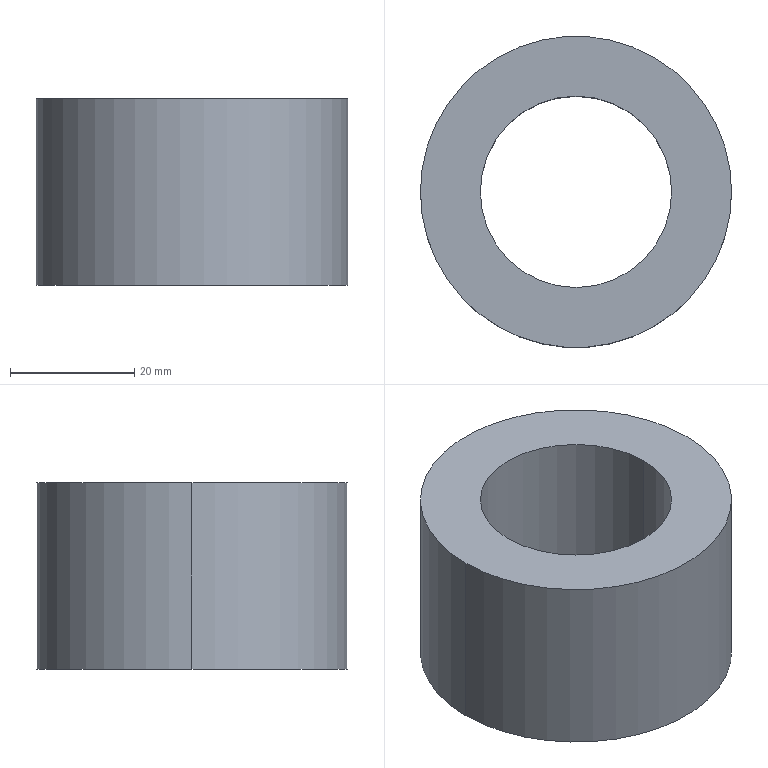Part | SolidWorks | features 3DProfileFeature 1, Extrusion 1, HoleWzd 1 | 1 solid | 6 faces | box 50 x 50 x 30 mm | volume 36626 mm3 | cylinder 4 | plane 2 | commonest cylinder face diameters 30.75 x2 50 x2
STEP:
#1=CARTESIAN_POINT('',(15.375,0.,30.));
#2=VERTEX_POINT('',#1);
#3=CARTESIAN_POINT('',(-15.375,0.,30.));
#4=VERTEX_POINT('',#3);
#5=CARTESIAN_POINT('',(0.,0.,30.));
#6=DIRECTION('',(0.,0.,-1.));
#7=DIRECTION('',(-1.,0.,0.));
#8=AXIS2_PLACEMENT_3D('',#5,#6,#7);
#9=CIRCLE('',#8,15.375);
#10=EDGE_CURVE('',#2,#4,#9,.T.);
#11=ORIENTED_EDGE('',*,*,#10,.F.);
#12=CARTESIAN_POINT('',(15.375,0.,0.));
#13=VERTEX_POINT('',#12);
#14=CARTESIAN_POINT('',(15.375,0.,0.));
#15=DIRECTION('',(0.,0.,-1.));
#16=VECTOR('',#15,1000.);
#17=LINE('',#14,#16);
#18=EDGE_CURVE('',#2,#13,#17,.T.);
#19=ORIENTED_EDGE('',*,*,#18,.T.);
#20=CARTESIAN_POINT('',(-15.375,0.,0.));
#21=VERTEX_POINT('',#20);
#22=CARTESIAN_POINT('',(0.,0.,0.));
#23=DIRECTION('',(0.,0.,-1.));
#24=DIRECTION('',(-1.,0.,0.));
#25=AXIS2_PLACEMENT_3D('',#22,#23,#24);
#26=CIRCLE('',#25,15.375);
#27=EDGE_CURVE('',#13,#21,#26,.T.);
#28=ORIENTED_EDGE('',*,*,#27,.T.);
#29=CARTESIAN_POINT('',(-15.375,0.,0.));
#30=DIRECTION('',(0.,0.,-1.));
#31=VECTOR('',#30,1000.);
#32=LINE('',#29,#31);
#33=EDGE_CURVE('',#4,#21,#32,.T.);
#34=ORIENTED_EDGE('',*,*,#33,.F.);
#35=EDGE_LOOP('',(#11,#19,#28,#34));
#36=FACE_OUTER_BOUND('',#35,.T.);
#37=CARTESIAN_POINT('',(0.,0.,0.));
#38=DIRECTION('',(0.,0.,-1.));
#39=DIRECTION('',(-1.,0.,0.));
#40=AXIS2_PLACEMENT_3D('',#37,#38,#39);
#41=CYLINDRICAL_SURFACE('',#40,15.375);
#42=ADVANCED_FACE('',(#36),#41,.F.);
#43=CARTESIAN_POINT('',(25.,0.,30.));
#44=VERTEX_POINT('',#43);
#45=CARTESIAN_POINT('',(-25.,0.,30.));
#46=VERTEX_POINT('',#45);
#47=CARTESIAN_POINT('',(0.,0.,30.));
#48=DIRECTION('',(0.,0.,1.));
#49=DIRECTION('',(1.,0.,0.));
#50=AXIS2_PLACEMENT_3D('',#47,#48,#49);
#51=CIRCLE('',#50,25.);
#52=EDGE_CURVE('',#44,#46,#51,.T.);
#53=ORIENTED_EDGE('',*,*,#52,.F.);
#54=CARTESIAN_POINT('',(25.,0.,0.));
#55=VERTEX_POINT('',#54);
#56=CARTESIAN_POINT('',(25.,0.,30.));
#57=DIRECTION('',(0.,0.,-1.));
#58=VECTOR('',#57,1000.);
#59=LINE('',#56,#58);
#60=EDGE_CURVE('',#44,#55,#59,.T.);
#61=ORIENTED_EDGE('',*,*,#60,.T.);
#62=CARTESIAN_POINT('',(-25.,0.,0.));
#63=VERTEX_POINT('',#62);
#64=CARTESIAN_POINT('',(0.,0.,0.));
#65=DIRECTION('',(0.,0.,1.));
#66=DIRECTION('',(1.,0.,0.));
#67=AXIS2_PLACEMENT_3D('',#64,#65,#66);
#68=CIRCLE('',#67,25.);
#69=EDGE_CURVE('',#55,#63,#68,.T.);
#70=ORIENTED_EDGE('',*,*,#69,.T.);
#71=CARTESIAN_POINT('',(-25.,0.,30.));
#72=DIRECTION('',(0.,0.,-1.));
#73=VECTOR('',#72,1000.);
#74=LINE('',#71,#73);
#75=EDGE_CURVE('',#46,#63,#74,.T.);
#76=ORIENTED_EDGE('',*,*,#75,.F.);
#77=EDGE_LOOP('',(#53,#61,#70,#76));
#78=FACE_OUTER_BOUND('',#77,.T.);
#79=CARTESIAN_POINT('',(0.,0.,30.));
#80=DIRECTION('',(0.,0.,-1.));
#81=DIRECTION('',(-1.,0.,0.));
#82=AXIS2_PLACEMENT_3D('',#79,#80,#81);
#83=CYLINDRICAL_SURFACE('',#82,25.);
#84=ADVANCED_FACE('',(#78),#83,.T.);
#85=ORIENTED_EDGE('',*,*,#60,.F.);
#86=CARTESIAN_POINT('',(0.,0.,30.));
#87=DIRECTION('',(0.,0.,1.));
#88=DIRECTION('',(1.,0.,0.));
#89=AXIS2_PLACEMENT_3D('',#86,#87,#88);
#90=CIRCLE('',#89,25.);
#91=EDGE_CURVE('',#46,#44,#90,.T.);
#92=ORIENTED_EDGE('',*,*,#91,.F.);
#93=ORIENTED_EDGE('',*,*,#75,.T.);
#94=CARTESIAN_POINT('',(0.,0.,0.));
#95=DIRECTION('',(0.,0.,1.));
#96=DIRECTION('',(1.,0.,0.));
#97=AXIS2_PLACEMENT_3D('',#94,#95,#96);
#98=CIRCLE('',#97,25.);
#99=EDGE_CURVE('',#63,#55,#98,.T.);
#100=ORIENTED_EDGE('',*,*,#99,.T.);
#101=EDGE_LOOP('',(#85,#92,#93,#100));
#102=FACE_OUTER_BOUND('',#101,.T.);
#103=CARTESIAN_POINT('',(0.,0.,30.));
#104=DIRECTION('',(0.,0.,-1.));
#105=DIRECTION('',(-1.,0.,0.));
#106=AXIS2_PLACEMENT_3D('',#103,#104,#105);
#107=CYLINDRICAL_SURFACE('',#106,25.);
#108=ADVANCED_FACE('',(#102),#107,.T.);
#109=CARTESIAN_POINT('',(0.,0.,30.));
#110=DIRECTION('',(0.,0.,-1.));
#111=DIRECTION('',(-1.,0.,0.));
#112=AXIS2_PLACEMENT_3D('',#109,#110,#111);
#113=CIRCLE('',#112,15.375);
#114=EDGE_CURVE('',#4,#2,#113,.T.);
#115=ORIENTED_EDGE('',*,*,#114,.T.);
#116=ORIENTED_EDGE('',*,*,#10,.T.);
#117=EDGE_LOOP('',(#115,#116));
#118=FACE_BOUND('',#117,.T.);
#119=ORIENTED_EDGE('',*,*,#91,.T.);
#120=ORIENTED_EDGE('',*,*,#52,.T.);
#121=EDGE_LOOP('',(#119,#120));
#122=FACE_OUTER_BOUND('',#121,.T.);
#123=CARTESIAN_POINT('',(0.,0.,30.));
#124=DIRECTION('',(0.,0.,1.));
#125=DIRECTION('',(1.,0.,0.));
#126=AXIS2_PLACEMENT_3D('',#123,#124,#125);
#127=PLANE('',#126);
#128=ADVANCED_FACE('',(#118,#122),#127,.T.);
#129=CARTESIAN_POINT('',(0.,0.,0.));
#130=DIRECTION('',(0.,0.,-1.));
#131=DIRECTION('',(-1.,0.,0.));
#132=AXIS2_PLACEMENT_3D('',#129,#130,#131);
#133=CIRCLE('',#132,15.375);
#134=EDGE_CURVE('',#21,#13,#133,.T.);
#135=ORIENTED_EDGE('',*,*,#134,.F.);
#136=ORIENTED_EDGE('',*,*,#27,.F.);
#137=EDGE_LOOP('',(#135,#136));
#138=FACE_BOUND('',#137,.T.);
#139=ORIENTED_EDGE('',*,*,#99,.F.);
#140=ORIENTED_EDGE('',*,*,#69,.F.);
#141=EDGE_LOOP('',(#139,#140));
#142=FACE_OUTER_BOUND('',#141,.T.);
#143=CARTESIAN_POINT('',(0.,0.,0.));
#144=DIRECTION('',(0.,0.,1.));
#145=DIRECTION('',(1.,0.,0.));
#146=AXIS2_PLACEMENT_3D('',#143,#144,#145);
#147=PLANE('',#146);
#148=ADVANCED_FACE('',(#138,#142),#147,.F.);
#149=ORIENTED_EDGE('',*,*,#18,.F.);
#150=ORIENTED_EDGE('',*,*,#114,.F.);
#151=ORIENTED_EDGE('',*,*,#33,.T.);
#152=ORIENTED_EDGE('',*,*,#134,.T.);
#153=EDGE_LOOP('',(#149,#150,#151,#152));
#154=FACE_OUTER_BOUND('',#153,.T.);
#155=CARTESIAN_POINT('',(0.,0.,0.));
#156=DIRECTION('',(0.,0.,-1.));
#157=DIRECTION('',(-1.,0.,0.));
#158=AXIS2_PLACEMENT_3D('',#155,#156,#157);
#159=CYLINDRICAL_SURFACE('',#158,15.375);
#160=ADVANCED_FACE('',(#154),#159,.F.);
#161=CLOSED_SHELL('',(#42,#84,#108,#128,#148,#160));
#162=MANIFOLD_SOLID_BREP('',#161);
#163=CARTESIAN_POINT('',(0.,0.,0.));
#164=DIRECTION('',(0.,0.,1.));
#165=DIRECTION('',(1.,0.,0.));
#166=AXIS2_PLACEMENT_3D('',#163,#164,#165);
#167=(LENGTH_UNIT()NAMED_UNIT(*)SI_UNIT(.MILLI.,.METRE.));
#168=UNCERTAINTY_MEASURE_WITH_UNIT(LENGTH_MEASURE(0.00001),#167,'','');
#169=(NAMED_UNIT(*)PLANE_ANGLE_UNIT()SI_UNIT($,.RADIAN.));
#170=(NAMED_UNIT(*)SI_UNIT($,.STERADIAN.)SOLID_ANGLE_UNIT());
#171=(GEOMETRIC_REPRESENTATION_CONTEXT(3)GLOBAL_UNCERTAINTY_ASSIGNED_CONTEXT((#168))GLOBAL_UNIT_ASSIGNED_CONTEXT((#167,#169,#170))REPRESENTATION_CONTEXT('',''));
#172=ADVANCED_BREP_SHAPE_REPRESENTATION('',(#162,#166),#171);